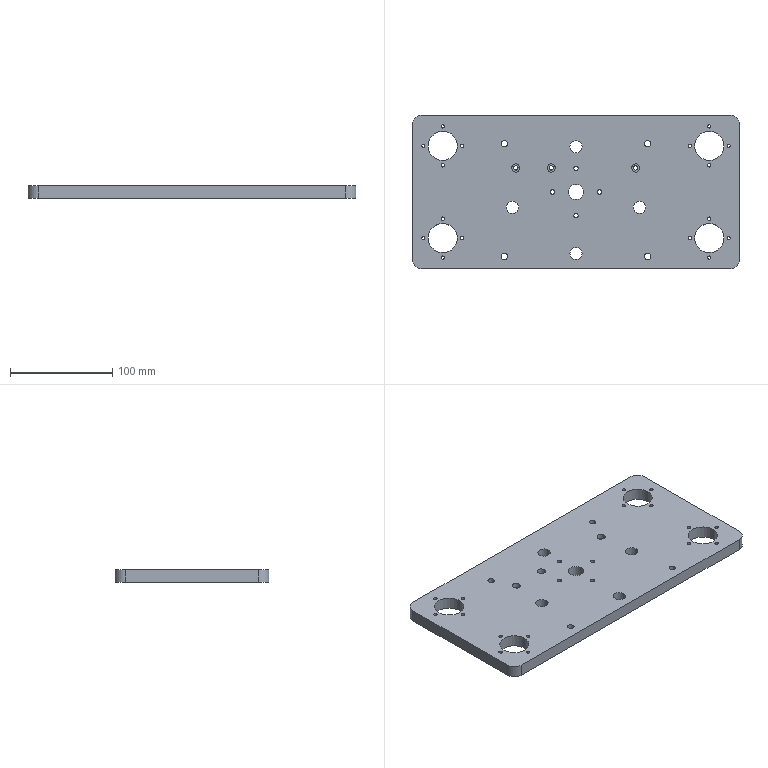Part | SolidWorks | features BaseBody 1 | 1 solid | 110 faces | box 320 x 150 x 12 mm | volume 530945 mm3 | cylinder 87 | plane 19 | spline 4 | commonest cylinder face diameters 3.3 x32 4.2 x14 6.2 x8 12 x8 28.5 x8 8 x6